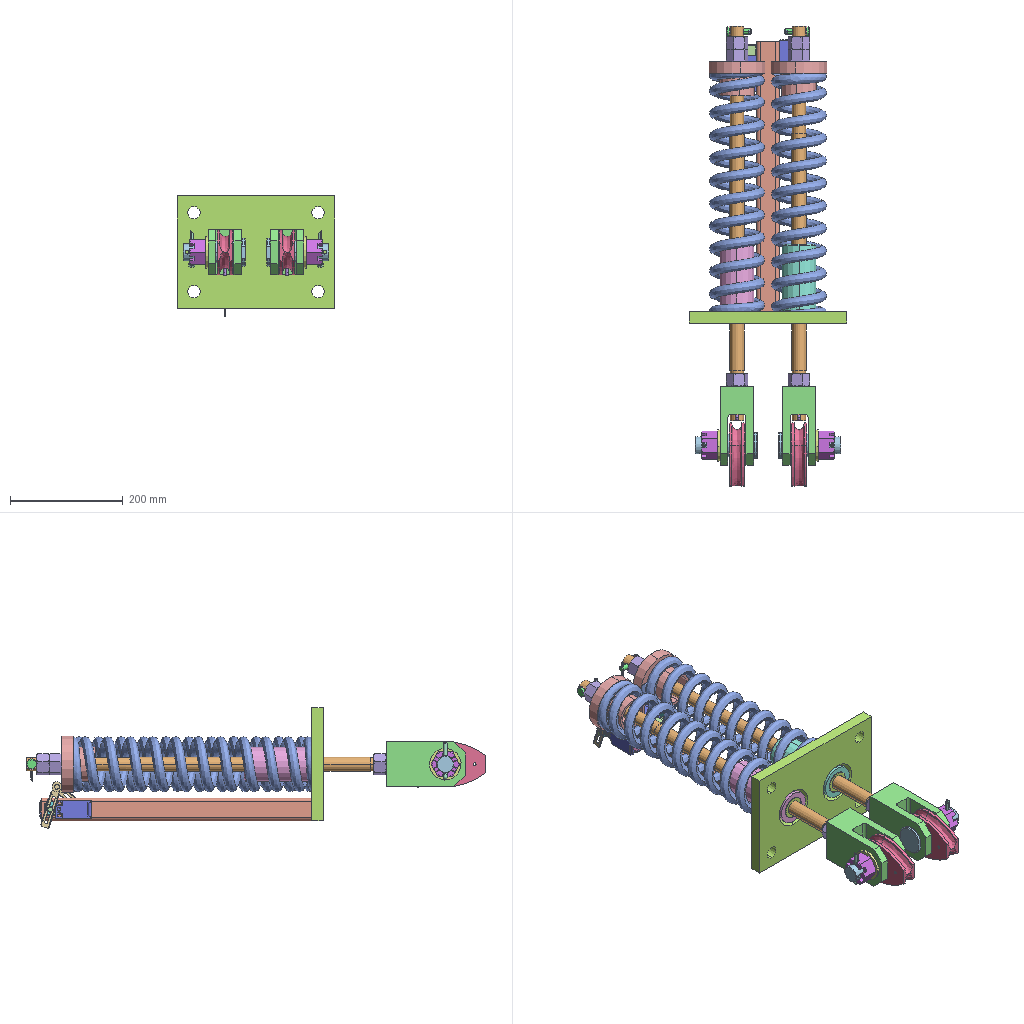Assembly | SolidWorks | 24 different items | 50 placed | box 280 x 815 x 213 mm
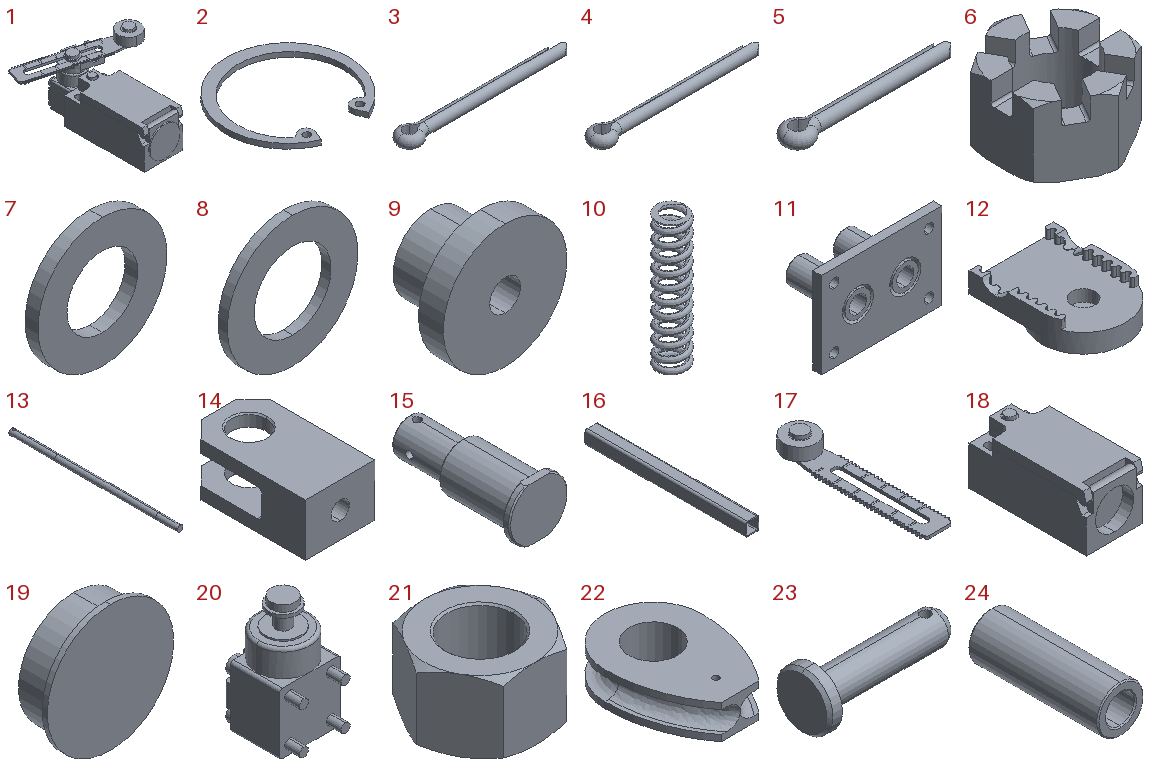Parts list (item | name | quantity | parent item | size | volume | features):
1 | (subassembly) | x2 | - | 82.59 x 90.924 x 45 mm | 70601 mm3 | -
2 | - | x2 | - | 43.5 x 41.844 x 1.75 mm | 670.953 mm3 | features Extrusion 1
3 | - | x2 | - | 41.6 x 5.8 x 2.9 mm | 263.569 mm3 | features ICE 1, Sweep 1
4 | - | x2 | - | 64 x 9.2 x 4.6 mm | 1032 mm3 | features ICE 1, Sweep 1
5 | - | x2 | - | 66.6 x 11.8 x 5.9 mm | 1774 mm3 | features ICE 1, Sweep 1
6 | - | x2 | - | 44.037 x 50.85 x 28.6 mm | 26766 mm3 | features Cut 3, Chamfer 1, CirPattern 1, Extrusion 1
7 | - | x2 | - | 20 x 2 x 20 mm | 438.252 mm3 | features Revolution 1
8 | - | x2 | - | 56 x 4 x 56 mm | 6431 mm3 | features Revolution 1
9 | - | x2 | - | 100 x 60 x 100 mm | 182448 mm3 | features Revolution 1
10 | - | x2 | - | 98 x 98 x 423 mm | 719372 mm3 | features Helix 1, ICE 1, RefAxis 1, Sweep 1
11 | - | x1 | - | 280 x 140 x 200 mm | 1375614 mm3 | features ICE 5, Chamfer 2, Extrusion 1, MirrorSolid 1
12 | - | x2 | in 1 | 18 x 24.5 x 5.9 mm | 1432 mm3 | features BaseBody 1
13 | - | x2 | - | 25 x 700 x 25 mm | 330452 mm3 | features ICE 4, Extrusion 1
14 | - | x2 | - | 80 x 140 x 60 mm | 378465 mm3 | features Chamfer 2, ICE 2, Extrusion 1, Fillet 1, HoleWzd 1
15 | - | x2 | - | 50 x 110 x 45 mm | 115257 mm3 | features ICE 3, Chamfer 1, Fillet 1, Revolution 1
16 | - | x1 | - | 40 x 480 x 40 mm | 201995 mm3 | features WeldMemberFeat 1, WeldmentFeature 1
17 | - | x2 | in 1 | 17.5 x 83.75 x 12 mm | 3070 mm3 | features BaseBody 1
18 | - | x2 | in 1 | 31 x 64 x 31.5 mm | 53225 mm3 | features BaseBody 1
19 | - | x2 | in 1 | 24 x 7 x 24 mm | 2522 mm3 | features BaseBody 1
20 | - | x2 | in 1 | 20.5 x 23.5 x 38.55 mm | 10352 mm3 | features BaseBody 1
21 | - | x6 | - | 39.6 x 34.295 x 22.3 mm | 15063 mm3 | features Cut 2, Chamfer 1, Extrusion 1
22 | - | x2 | - | 80 x 112 x 28 mm | 116834 mm3 | features Extrusion 1, SweepCut 1
23 | - | x2 | - | 44 x 18 x 18 mm | 4022 mm3 | features Chamfer 1, Fillet 1, ICE 1, Revolution 1
24 | - | x2 | - | 40 x 112 x 40 mm | 85561 mm3 | features Chamfer 1, Extrusion 1
Mates (type | each side: item.copy, entity, surface, feature):
In the top assembly
Coordinate | 11.1 select_type:25 | assembly select_type:11
Concentric | 11.1 face cylinder Cut-Extrude2 | 13.1 face cylinder Boss-Extrude3
Coincident | 10.1 face plane Cut-Extrude1 | 11.1 face plane Boss-Extrude2
Concentric | 10.1 axis | 11.1 face cylinder Boss-Extrude5
Concentric | 11.1 face cylinder Cut-Extrude3 | 24.1 face cylinder Boss-Extrude1
Coincident | 11.1 face plane Boss-Extrude5 | 24.1 face plane Boss-Extrude1
Concentric | 13.1 face cylinder Boss-Extrude1 | 14.1 face cylinder M24 Tapped Hole1
Concentric | 13.1 face cylinder Boss-Extrude1 | 21.1 face cylinder Base-Extrude
Coincident | 14.1 face plane Boss-Extrude1 | 21.1 face plane Base-Extrude
DistanceDim | 21.1 face plane Base-Extrude | 13.1 face plane Boss-Extrude2
Concentric | 14.1 face cylinder Cut-Extrude2 | 15.1 face cylinder Revolve1
Coincident | 14.1 face plane Boss-Extrude1 | 15.1 face plane Revolve1
Parallel | 14.1 face plane Boss-Extrude1 | 15.1 face plane Cut-Extrude1
Concentric | 15.1 face cylinder Revolve1 | 6.1 face cylinder Base-Extrude
Parallel | 14.1 face plane Boss-Extrude1 | 6.1 face plane Base-Extrude
Concentric | 15.1 face cylinder Revolve1 | 8.1 face cylinder Base-Revolve
Coincident | 14.1 face plane Boss-Extrude1 | 8.1 face plane Base-Revolve
Coincident | 6.1 face plane Base-Extrude | 8.1 face plane Base-Revolve
Concentric | 15.1 face cylinder Cut-Extrude3 | 5.1 face cylinder Sweep2
Tangent | 15.1 face cylinder Revolve1 | 5.1 edge
Concentric | 15.1 face cylinder Revolve1 | 22.1 face cylinder Boss-Extrude1
DistanceDim | 22.1 face plane Boss-Extrude1 | 14.1 face plane Cut-Extrude1
Parallel | 14.1 face plane Boss-Extrude1 | assembly plane
Parallel | 22.1 plane | assembly plane
Concentric | 9.1 face cylinder Revolve1 | 13.1 face cylinder Boss-Extrude3
Coincident | 9.1 face plane Revolve1 | 10.1 face plane Cut-Extrude1
Concentric | 21.2 face cylinder Base-Extrude | 21.3 face cylinder Base-Extrude
Coincident | 21.2 face plane Base-Extrude | 21.3 face plane Base-Extrude | 2 times
Coincident | 21.1 face plane Base-Extrude | 21.2 face plane Base-Extrude
Concentric | 13.1 face cylinder Boss-Extrude3 | 21.3 face cylinder Base-Extrude
Coincident | 9.1 face plane Revolve1 | 21.3 face plane Base-Extrude
Coincident | 11.1 face plane Boss-Extrude2 | 16.1 face plane Cold-formed hollow square steel (gb t6728-2002) 40×3-example.com(1) | 2 times
Width | 16.1 face plane Cold-formed hollow square steel (gb t6728-2002) 40×3-example.com(1) | 16.1 face plane Cold-formed hollow square steel (gb t6728-2002) 40×3-example.com(1) | 11.1 face plane Boss-Extrude2 | 11.1 face plane Boss-Extrude2
Coincident | 16.1 face plane Cold-formed hollow square steel (gb t6728-2002) 40×3-example.com(1) | 18.1 face plane Imported1
Width | 16.1 face plane Cold-formed hollow square steel (gb t6728-2002) 40×3-example.com(1) | 16.1 face plane Cold-formed hollow square steel (gb t6728-2002) 40×3-example.com(1) | 18.1 face plane Imported1 | 18.1 face plane Imported1
DistanceDim | 18.1 face plane Imported1 | 16.1 face plane Cold-formed hollow square steel (gb t6728-2002) 40×3-example.com(1)
Parallel | 5.1 face plane Sweep2 | 6.1 face plane Base-Extrude
Tangent | 9.1 face plane Revolve1 | 17.1 face cylinder Imported1
Concentric | 17.1 face cylinder Imported1 | 17.2 face cylinder Imported1
PlanarAngleDim | 17.1 face plane Imported1 | 16.1 face plane Cold-formed hollow square steel (gb t6728-2002) 40×3-example.com(1)
Concentric | 13.1 face cylinder Cut-Extrude1 | 23.1 face cylinder Base-Revolve
Parallel | 13.1 plane | assembly plane
Concentric | 3.1 face cylinder Sweep2 | 23.1 face cylinder Cut-Extrude1
Parallel | 13.1 face plane Boss-Extrude3 | 3.1 face plane Sweep2
Tangent | 3.1 edge | 23.1 face cylinder Base-Revolve
Concentric | 13.1 face cylinder Cut-Extrude2 | 4.1 face cylinder Sweep2
Tangent | 13.1 face cylinder Boss-Extrude1 | 4.1 edge
Parallel | 14.1 face plane Boss-Extrude1 | 4.1 face plane Sweep2
Concentric | 23.1 face cylinder Base-Revolve | 7.1 face cylinder Base-Revolve
Coincident | 23.1 face plane Base-Revolve | 7.1 face plane Base-Revolve
Tangent | 13.1 face cylinder Boss-Extrude3 | 7.1 face plane Base-Revolve
Concentric | 11.1 face cylinder Cut-Extrude5 | 2.1 face cylinder Base-Extrude
Coincident | 24.1 face plane Boss-Extrude1 | 2.1 face plane Base-Extrude
In subassembly 1
Concentric | 18.2 face cylinder Imported1 | 20.1 face cylinder Imported1 | 2 times
Coincident | 18.2 face plane Imported1 | 20.1 face plane Imported1
Coincident | 18.2 face plane Imported1 | 19.1 face plane Imported1
Concentric | 18.2 face cylinder Imported1 | 19.1 face cylinder Imported1
Parallel | 19.1 plane | 1.1 plane
Coincident | 20.1 face plane Imported1 | 12.1 face plane Imported1
Concentric | 20.1 face cylinder Imported1 | 12.1 face cylinder Imported1
Coincident | 12.1 face plane Imported1 | 17.3 face plane Imported1
Coincident | 12.1 plane | 17.3 plane